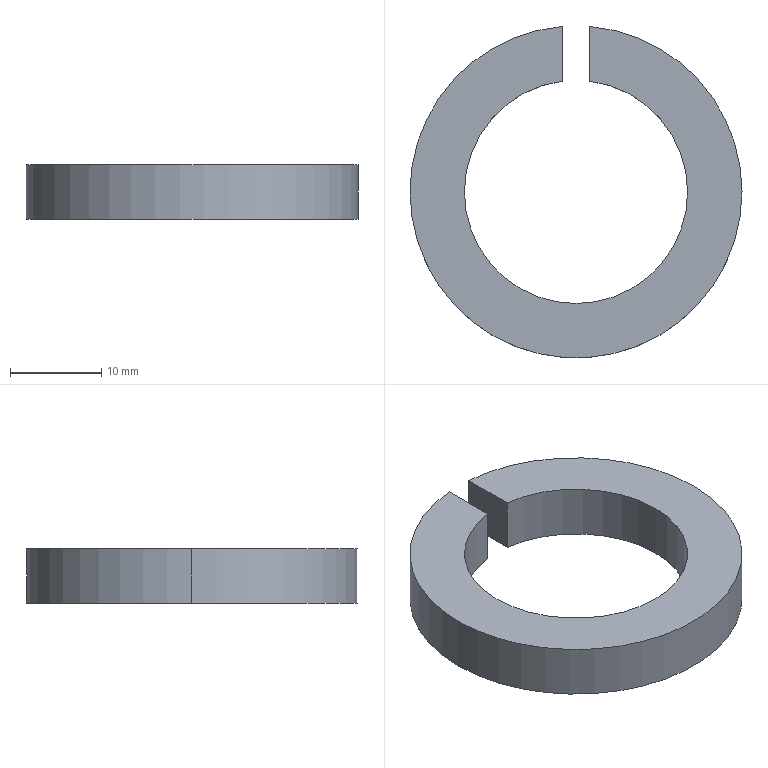Part | STEP file | GB/T 93-1987 standard spring washer (assembly) 24×6 (65Mn) | 1 solid | 10 faces | box 36.439 x 36.377 x 6 mm | volume 3321 mm3 | cylinder 6 | plane 4 | commonest cylinder face diameters 24.5 x3 36.439 x3
STEP:
#1=CARTESIAN_POINT('',(0.,0.,0.));
#2=DIRECTION('',(0.,0.,1.));
#3=DIRECTION('',(1.,0.,0.));
#4=AXIS2_PLACEMENT_3D('',#1,#2,#3);
#5=CARTESIAN_POINT('',(-12.25,0.,6.));
#6=VERTEX_POINT('',#5);
#7=CARTESIAN_POINT('',(-12.25,0.,0.));
#8=VERTEX_POINT('',#7);
#9=CARTESIAN_POINT('',(-12.25,0.,6.));
#10=DIRECTION('',(0.,0.,-1.));
#11=VECTOR('',#10,1.);
#12=LINE('',#9,#11);
#13=CARTESIAN_POINT('',(0.,0.,6.));
#14=DIRECTION('',(0.,0.,-1.));
#15=DIRECTION('',(-1.,0.,0.));
#16=AXIS2_PLACEMENT_3D('',#13,#14,#15);
#17=CYLINDRICAL_SURFACE('',#16,12.25);
#18=CARTESIAN_POINT('',(6.283,0.));
#19=DIRECTION('',(0.,1.));
#20=VECTOR('',#19,1.);
#21=LINE('',#18,#20);
#22=(GEOMETRIC_REPRESENTATION_CONTEXT(2)PARAMETRIC_REPRESENTATION_CONTEXT()REPRESENTATION_CONTEXT('',''));
#23=DEFINITIONAL_REPRESENTATION('',(#21),#22);
#24=PCURVE('',#17,#23);
#25=CARTESIAN_POINT('',(0.,0.,6.));
#26=DIRECTION('',(0.,0.,-1.));
#27=DIRECTION('',(-1.,0.,0.));
#28=AXIS2_PLACEMENT_3D('',#25,#26,#27);
#29=CYLINDRICAL_SURFACE('',#28,12.25);
#30=CARTESIAN_POINT('',(0.,0.));
#31=DIRECTION('',(0.,1.));
#32=VECTOR('',#31,1.);
#33=LINE('',#30,#32);
#34=(GEOMETRIC_REPRESENTATION_CONTEXT(2)PARAMETRIC_REPRESENTATION_CONTEXT()REPRESENTATION_CONTEXT('',''));
#35=DEFINITIONAL_REPRESENTATION('',(#33),#34);
#36=PCURVE('',#29,#35);
#37=SURFACE_CURVE('',#12,(#24,#36),.PCURVE_S1.);
#38=EDGE_CURVE('',#6,#8,#37,.T.);
#39=ORIENTED_EDGE('',*,*,#38,.T.);
#40=CARTESIAN_POINT('',(12.25,0.,0.));
#41=VERTEX_POINT('',#40);
#42=CARTESIAN_POINT('',(0.,0.,0.));
#43=DIRECTION('',(0.,0.,-1.));
#44=DIRECTION('',(1.,0.,0.));
#45=AXIS2_PLACEMENT_3D('',#42,#43,#44);
#46=CIRCLE('',#45,12.25);
#47=CARTESIAN_POINT('',(3.142,6.));
#48=DIRECTION('',(1.,0.));
#49=VECTOR('',#48,1.);
#50=LINE('',#47,#49);
#51=(GEOMETRIC_REPRESENTATION_CONTEXT(2)PARAMETRIC_REPRESENTATION_CONTEXT()REPRESENTATION_CONTEXT('',''));
#52=DEFINITIONAL_REPRESENTATION('',(#50),#51);
#53=PCURVE('',#17,#52);
#54=CARTESIAN_POINT('',(0.,0.,0.));
#55=DIRECTION('',(0.,0.,1.));
#56=DIRECTION('',(1.,0.,0.));
#57=AXIS2_PLACEMENT_3D('',#54,#55,#56);
#58=PLANE('',#57);
#59=CARTESIAN_POINT('',(12.25,0.));
#60=CARTESIAN_POINT('',(12.25,-21.218));
#61=CARTESIAN_POINT('',(-6.125,-10.609));
#62=CARTESIAN_POINT('',(-24.5,0.));
#63=CARTESIAN_POINT('',(-6.125,10.609));
#64=CARTESIAN_POINT('',(12.25,21.218));
#65=CARTESIAN_POINT('',(12.25,0.));
#66=(BOUNDED_CURVE()B_SPLINE_CURVE(2,(#59,#60,#61,#62,#63,#64,#65),.UNSPECIFIED.,.T.,.F.)B_SPLINE_CURVE_WITH_KNOTS((1,2,2,2,2,1),(-2.094,0.,2.094,4.189,6.283,8.378),.UNSPECIFIED.)CURVE()GEOMETRIC_REPRESENTATION_ITEM()RATIONAL_B_SPLINE_CURVE((1.,0.5,1.,0.5,1.,0.5,1.))REPRESENTATION_ITEM(''));
#67=(GEOMETRIC_REPRESENTATION_CONTEXT(2)PARAMETRIC_REPRESENTATION_CONTEXT()REPRESENTATION_CONTEXT('',''));
#68=DEFINITIONAL_REPRESENTATION('',(#66),#67);
#69=PCURVE('',#58,#68);
#70=SURFACE_CURVE('',#46,(#53,#69),.PCURVE_S1.);
#71=EDGE_CURVE('',#41,#8,#70,.T.);
#72=ORIENTED_EDGE('',*,*,#71,.F.);
#73=CARTESIAN_POINT('',(12.25,0.,6.));
#74=VERTEX_POINT('',#73);
#75=CARTESIAN_POINT('',(12.25,0.,6.));
#76=DIRECTION('',(0.,0.,-1.));
#77=VECTOR('',#76,1.);
#78=LINE('',#75,#77);
#79=CARTESIAN_POINT('',(3.142,0.));
#80=DIRECTION('',(0.,1.));
#81=VECTOR('',#80,1.);
#82=LINE('',#79,#81);
#83=(GEOMETRIC_REPRESENTATION_CONTEXT(2)PARAMETRIC_REPRESENTATION_CONTEXT()REPRESENTATION_CONTEXT('',''));
#84=DEFINITIONAL_REPRESENTATION('',(#82),#83);
#85=PCURVE('',#17,#84);
#86=CARTESIAN_POINT('',(0.,0.,6.));
#87=DIRECTION('',(0.,0.,-1.));
#88=DIRECTION('',(-1.,0.,0.));
#89=AXIS2_PLACEMENT_3D('',#86,#87,#88);
#90=CYLINDRICAL_SURFACE('',#89,12.25);
#91=CARTESIAN_POINT('',(3.142,0.));
#92=DIRECTION('',(0.,1.));
#93=VECTOR('',#92,1.);
#94=LINE('',#91,#93);
#95=(GEOMETRIC_REPRESENTATION_CONTEXT(2)PARAMETRIC_REPRESENTATION_CONTEXT()REPRESENTATION_CONTEXT('',''));
#96=DEFINITIONAL_REPRESENTATION('',(#94),#95);
#97=PCURVE('',#90,#96);
#98=SURFACE_CURVE('',#78,(#85,#97),.PCURVE_S1.);
#99=EDGE_CURVE('',#74,#41,#98,.T.);
#100=ORIENTED_EDGE('',*,*,#99,.F.);
#101=CARTESIAN_POINT('',(0.,0.,6.));
#102=DIRECTION('',(0.,0.,-1.));
#103=DIRECTION('',(1.,0.,0.));
#104=AXIS2_PLACEMENT_3D('',#101,#102,#103);
#105=CIRCLE('',#104,12.25);
#106=CARTESIAN_POINT('',(3.142,0.));
#107=DIRECTION('',(1.,0.));
#108=VECTOR('',#107,1.);
#109=LINE('',#106,#108);
#110=(GEOMETRIC_REPRESENTATION_CONTEXT(2)PARAMETRIC_REPRESENTATION_CONTEXT()REPRESENTATION_CONTEXT('',''));
#111=DEFINITIONAL_REPRESENTATION('',(#109),#110);
#112=PCURVE('',#17,#111);
#113=CARTESIAN_POINT('',(0.,0.,6.));
#114=DIRECTION('',(0.,0.,1.));
#115=DIRECTION('',(1.,0.,0.));
#116=AXIS2_PLACEMENT_3D('',#113,#114,#115);
#117=PLANE('',#116);
#118=CARTESIAN_POINT('',(12.25,0.));
#119=CARTESIAN_POINT('',(12.25,-21.218));
#120=CARTESIAN_POINT('',(-6.125,-10.609));
#121=CARTESIAN_POINT('',(-24.5,0.));
#122=CARTESIAN_POINT('',(-6.125,10.609));
#123=CARTESIAN_POINT('',(12.25,21.218));
#124=CARTESIAN_POINT('',(12.25,0.));
#125=(BOUNDED_CURVE()B_SPLINE_CURVE(2,(#118,#119,#120,#121,#122,#123,#124),.UNSPECIFIED.,.T.,.F.)B_SPLINE_CURVE_WITH_KNOTS((1,2,2,2,2,1),(-2.094,0.,2.094,4.189,6.283,8.378),.UNSPECIFIED.)CURVE()GEOMETRIC_REPRESENTATION_ITEM()RATIONAL_B_SPLINE_CURVE((1.,0.5,1.,0.5,1.,0.5,1.))REPRESENTATION_ITEM(''));
#126=(GEOMETRIC_REPRESENTATION_CONTEXT(2)PARAMETRIC_REPRESENTATION_CONTEXT()REPRESENTATION_CONTEXT('',''));
#127=DEFINITIONAL_REPRESENTATION('',(#125),#126);
#128=PCURVE('',#117,#127);
#129=SURFACE_CURVE('',#105,(#112,#128),.PCURVE_S1.);
#130=EDGE_CURVE('',#74,#6,#129,.T.);
#131=ORIENTED_EDGE('',*,*,#130,.T.);
#132=EDGE_LOOP('',(#39,#72,#100,#131));
#133=FACE_BOUND('',#132,.F.);
#134=ADVANCED_FACE('',(#133),#17,.F.);
#135=CARTESIAN_POINT('',(-1.5,12.158,6.));
#136=VERTEX_POINT('',#135);
#137=CARTESIAN_POINT('',(-1.5,12.158,0.));
#138=VERTEX_POINT('',#137);
#139=CARTESIAN_POINT('',(-1.5,12.158,6.));
#140=DIRECTION('',(0.,0.,-1.));
#141=VECTOR('',#140,1.);
#142=LINE('',#139,#141);
#143=CARTESIAN_POINT('',(1.448,0.));
#144=DIRECTION('',(0.,1.));
#145=VECTOR('',#144,1.);
#146=LINE('',#143,#145);
#147=(GEOMETRIC_REPRESENTATION_CONTEXT(2)PARAMETRIC_REPRESENTATION_CONTEXT()REPRESENTATION_CONTEXT('',''));
#148=DEFINITIONAL_REPRESENTATION('',(#146),#147);
#149=PCURVE('',#29,#148);
#150=CARTESIAN_POINT('',(-1.5,18.158,6.));
#151=DIRECTION('',(-1.,0.,0.));
#152=DIRECTION('',(0.,0.,1.));
#153=AXIS2_PLACEMENT_3D('',#150,#151,#152);
#154=PLANE('',#153);
#155=CARTESIAN_POINT('',(0.,-6.));
#156=DIRECTION('',(-1.,0.));
#157=VECTOR('',#156,1.);
#158=LINE('',#155,#157);
#159=(GEOMETRIC_REPRESENTATION_CONTEXT(2)PARAMETRIC_REPRESENTATION_CONTEXT()REPRESENTATION_CONTEXT('',''));
#160=DEFINITIONAL_REPRESENTATION('',(#158),#159);
#161=PCURVE('',#154,#160);
#162=SURFACE_CURVE('',#142,(#149,#161),.PCURVE_S1.);
#163=EDGE_CURVE('',#136,#138,#162,.T.);
#164=ORIENTED_EDGE('',*,*,#163,.T.);
#165=CARTESIAN_POINT('',(0.,0.,0.));
#166=DIRECTION('',(0.,0.,-1.));
#167=DIRECTION('',(1.,0.,0.));
#168=AXIS2_PLACEMENT_3D('',#165,#166,#167);
#169=CIRCLE('',#168,12.25);
#170=CARTESIAN_POINT('',(-3.142,6.));
#171=DIRECTION('',(1.,0.));
#172=VECTOR('',#171,1.);
#173=LINE('',#170,#172);
#174=(GEOMETRIC_REPRESENTATION_CONTEXT(2)PARAMETRIC_REPRESENTATION_CONTEXT()REPRESENTATION_CONTEXT('',''));
#175=DEFINITIONAL_REPRESENTATION('',(#173),#174);
#176=PCURVE('',#29,#175);
#177=CARTESIAN_POINT('',(12.25,0.));
#178=CARTESIAN_POINT('',(12.25,-21.218));
#179=CARTESIAN_POINT('',(-6.125,-10.609));
#180=CARTESIAN_POINT('',(-24.5,0.));
#181=CARTESIAN_POINT('',(-6.125,10.609));
#182=CARTESIAN_POINT('',(12.25,21.218));
#183=CARTESIAN_POINT('',(12.25,0.));
#184=(BOUNDED_CURVE()B_SPLINE_CURVE(2,(#177,#178,#179,#180,#181,#182,#183),.UNSPECIFIED.,.T.,.F.)B_SPLINE_CURVE_WITH_KNOTS((1,2,2,2,2,1),(-2.094,0.,2.094,4.189,6.283,8.378),.UNSPECIFIED.)CURVE()GEOMETRIC_REPRESENTATION_ITEM()RATIONAL_B_SPLINE_CURVE((1.,0.5,1.,0.5,1.,0.5,1.))REPRESENTATION_ITEM(''));
#185=(GEOMETRIC_REPRESENTATION_CONTEXT(2)PARAMETRIC_REPRESENTATION_CONTEXT()REPRESENTATION_CONTEXT('',''));
#186=DEFINITIONAL_REPRESENTATION('',(#184),#185);
#187=PCURVE('',#58,#186);
#188=SURFACE_CURVE('',#169,(#176,#187),.PCURVE_S1.);
#189=EDGE_CURVE('',#8,#138,#188,.T.);
#190=ORIENTED_EDGE('',*,*,#189,.F.);
#191=ORIENTED_EDGE('',*,*,#38,.F.);
#192=CARTESIAN_POINT('',(0.,0.,6.));
#193=DIRECTION('',(0.,0.,-1.));
#194=DIRECTION('',(1.,0.,0.));
#195=AXIS2_PLACEMENT_3D('',#192,#193,#194);
#196=CIRCLE('',#195,12.25);
#197=CARTESIAN_POINT('',(-3.142,0.));
#198=DIRECTION('',(1.,0.));
#199=VECTOR('',#198,1.);
#200=LINE('',#197,#199);
#201=(GEOMETRIC_REPRESENTATION_CONTEXT(2)PARAMETRIC_REPRESENTATION_CONTEXT()REPRESENTATION_CONTEXT('',''));
#202=DEFINITIONAL_REPRESENTATION('',(#200),#201);
#203=PCURVE('',#29,#202);
#204=CARTESIAN_POINT('',(12.25,0.));
#205=CARTESIAN_POINT('',(12.25,-21.218));
#206=CARTESIAN_POINT('',(-6.125,-10.609));
#207=CARTESIAN_POINT('',(-24.5,0.));
#208=CARTESIAN_POINT('',(-6.125,10.609));
#209=CARTESIAN_POINT('',(12.25,21.218));
#210=CARTESIAN_POINT('',(12.25,0.));
#211=(BOUNDED_CURVE()B_SPLINE_CURVE(2,(#204,#205,#206,#207,#208,#209,#210),.UNSPECIFIED.,.T.,.F.)B_SPLINE_CURVE_WITH_KNOTS((1,2,2,2,2,1),(-2.094,0.,2.094,4.189,6.283,8.378),.UNSPECIFIED.)CURVE()GEOMETRIC_REPRESENTATION_ITEM()RATIONAL_B_SPLINE_CURVE((1.,0.5,1.,0.5,1.,0.5,1.))REPRESENTATION_ITEM(''));
#212=(GEOMETRIC_REPRESENTATION_CONTEXT(2)PARAMETRIC_REPRESENTATION_CONTEXT()REPRESENTATION_CONTEXT('',''));
#213=DEFINITIONAL_REPRESENTATION('',(#211),#212);
#214=PCURVE('',#117,#213);
#215=SURFACE_CURVE('',#196,(#203,#214),.PCURVE_S1.);
#216=EDGE_CURVE('',#6,#136,#215,.T.);
#217=ORIENTED_EDGE('',*,*,#216,.T.);
#218=EDGE_LOOP('',(#164,#190,#191,#217));
#219=FACE_BOUND('',#218,.F.);
#220=ADVANCED_FACE('',(#219),#29,.F.);
#221=CARTESIAN_POINT('',(18.22,0.,6.));
#222=VERTEX_POINT('',#221);
#223=CARTESIAN_POINT('',(1.5,18.158,6.));
#224=VERTEX_POINT('',#223);
#225=CARTESIAN_POINT('',(0.,0.,6.));
#226=DIRECTION('',(0.,0.,1.));
#227=DIRECTION('',(1.,0.,0.));
#228=AXIS2_PLACEMENT_3D('',#225,#226,#227);
#229=CIRCLE('',#228,18.22);
#230=CARTESIAN_POINT('',(0.,0.,6.));
#231=DIRECTION('',(0.,0.,-1.));
#232=DIRECTION('',(-1.,0.,0.));
#233=AXIS2_PLACEMENT_3D('',#230,#231,#232);
#234=CYLINDRICAL_SURFACE('',#233,18.22);
#235=CARTESIAN_POINT('',(3.142,0.));
#236=DIRECTION('',(-1.,0.));
#237=VECTOR('',#236,1.);
#238=LINE('',#235,#237);
#239=(GEOMETRIC_REPRESENTATION_CONTEXT(2)PARAMETRIC_REPRESENTATION_CONTEXT()REPRESENTATION_CONTEXT('',''));
#240=DEFINITIONAL_REPRESENTATION('',(#238),#239);
#241=PCURVE('',#234,#240);
#242=CARTESIAN_POINT('',(0.,0.));
#243=DIRECTION('',(1.,0.));
#244=AXIS2_PLACEMENT_2D('',#242,#243);
#245=CIRCLE('',#244,18.22);
#246=(GEOMETRIC_REPRESENTATION_CONTEXT(2)PARAMETRIC_REPRESENTATION_CONTEXT()REPRESENTATION_CONTEXT('',''));
#247=DEFINITIONAL_REPRESENTATION('',(#245),#246);
#248=PCURVE('',#117,#247);
#249=SURFACE_CURVE('',#229,(#241,#248),.PCURVE_S1.);
#250=EDGE_CURVE('',#222,#224,#249,.T.);
#251=ORIENTED_EDGE('',*,*,#250,.F.);
#252=CARTESIAN_POINT('',(18.22,0.,0.));
#253=VERTEX_POINT('',#252);
#254=CARTESIAN_POINT('',(18.22,0.,6.));
#255=DIRECTION('',(0.,0.,-1.));
#256=VECTOR('',#255,1.);
#257=LINE('',#254,#256);
#258=CARTESIAN_POINT('',(3.142,0.));
#259=DIRECTION('',(0.,1.));
#260=VECTOR('',#259,1.);
#261=LINE('',#258,#260);
#262=(GEOMETRIC_REPRESENTATION_CONTEXT(2)PARAMETRIC_REPRESENTATION_CONTEXT()REPRESENTATION_CONTEXT('',''));
#263=DEFINITIONAL_REPRESENTATION('',(#261),#262);
#264=PCURVE('',#234,#263);
#265=CARTESIAN_POINT('',(0.,0.,6.));
#266=DIRECTION('',(0.,0.,-1.));
#267=DIRECTION('',(-1.,0.,0.));
#268=AXIS2_PLACEMENT_3D('',#265,#266,#267);
#269=CYLINDRICAL_SURFACE('',#268,18.22);
#270=CARTESIAN_POINT('',(3.142,0.));
#271=DIRECTION('',(0.,1.));
#272=VECTOR('',#271,1.);
#273=LINE('',#270,#272);
#274=(GEOMETRIC_REPRESENTATION_CONTEXT(2)PARAMETRIC_REPRESENTATION_CONTEXT()REPRESENTATION_CONTEXT('',''));
#275=DEFINITIONAL_REPRESENTATION('',(#273),#274);
#276=PCURVE('',#269,#275);
#277=SURFACE_CURVE('',#257,(#264,#276),.PCURVE_S1.);
#278=EDGE_CURVE('',#222,#253,#277,.T.);
#279=ORIENTED_EDGE('',*,*,#278,.T.);
#280=CARTESIAN_POINT('',(1.5,18.158,0.));
#281=VERTEX_POINT('',#280);
#282=CARTESIAN_POINT('',(0.,0.,0.));
#283=DIRECTION('',(0.,0.,1.));
#284=DIRECTION('',(1.,0.,0.));
#285=AXIS2_PLACEMENT_3D('',#282,#283,#284);
#286=CIRCLE('',#285,18.22);
#287=CARTESIAN_POINT('',(3.142,6.));
#288=DIRECTION('',(-1.,0.));
#289=VECTOR('',#288,1.);
#290=LINE('',#287,#289);
#291=(GEOMETRIC_REPRESENTATION_CONTEXT(2)PARAMETRIC_REPRESENTATION_CONTEXT()REPRESENTATION_CONTEXT('',''));
#292=DEFINITIONAL_REPRESENTATION('',(#290),#291);
#293=PCURVE('',#234,#292);
#294=CARTESIAN_POINT('',(0.,0.));
#295=DIRECTION('',(1.,0.));
#296=AXIS2_PLACEMENT_2D('',#294,#295);
#297=CIRCLE('',#296,18.22);
#298=(GEOMETRIC_REPRESENTATION_CONTEXT(2)PARAMETRIC_REPRESENTATION_CONTEXT()REPRESENTATION_CONTEXT('',''));
#299=DEFINITIONAL_REPRESENTATION('',(#297),#298);
#300=PCURVE('',#58,#299);
#301=SURFACE_CURVE('',#286,(#293,#300),.PCURVE_S1.);
#302=EDGE_CURVE('',#253,#281,#301,.T.);
#303=ORIENTED_EDGE('',*,*,#302,.T.);
#304=CARTESIAN_POINT('',(1.5,18.158,6.));
#305=DIRECTION('',(0.,0.,-1.));
#306=VECTOR('',#305,1.);
#307=LINE('',#304,#306);
#308=CARTESIAN_POINT('',(1.653,0.));
#309=DIRECTION('',(0.,1.));
#310=VECTOR('',#309,1.);
#311=LINE('',#308,#310);
#312=(GEOMETRIC_REPRESENTATION_CONTEXT(2)PARAMETRIC_REPRESENTATION_CONTEXT()REPRESENTATION_CONTEXT('',''));
#313=DEFINITIONAL_REPRESENTATION('',(#311),#312);
#314=PCURVE('',#234,#313);
#315=CARTESIAN_POINT('',(1.5,18.158,6.));
#316=DIRECTION('',(1.,0.,0.));
#317=DIRECTION('',(0.,0.,-1.));
#318=AXIS2_PLACEMENT_3D('',#315,#316,#317);
#319=PLANE('',#318);
#320=CARTESIAN_POINT('',(0.,0.));
#321=DIRECTION('',(1.,0.));
#322=VECTOR('',#321,1.);
#323=LINE('',#320,#322);
#324=(GEOMETRIC_REPRESENTATION_CONTEXT(2)PARAMETRIC_REPRESENTATION_CONTEXT()REPRESENTATION_CONTEXT('',''));
#325=DEFINITIONAL_REPRESENTATION('',(#323),#324);
#326=PCURVE('',#319,#325);
#327=SURFACE_CURVE('',#307,(#314,#326),.PCURVE_S1.);
#328=EDGE_CURVE('',#224,#281,#327,.T.);
#329=ORIENTED_EDGE('',*,*,#328,.F.);
#330=EDGE_LOOP('',(#251,#279,#303,#329));
#331=FACE_BOUND('',#330,.T.);
#332=ADVANCED_FACE('',(#331),#234,.T.);
#333=ORIENTED_EDGE('',*,*,#278,.F.);
#334=CARTESIAN_POINT('',(-18.22,0.,6.));
#335=VERTEX_POINT('',#334);
#336=CARTESIAN_POINT('',(0.,0.,6.));
#337=DIRECTION('',(0.,0.,1.));
#338=DIRECTION('',(1.,0.,0.));
#339=AXIS2_PLACEMENT_3D('',#336,#337,#338);
#340=CIRCLE('',#339,18.22);
#341=CARTESIAN_POINT('',(9.425,0.));
#342=DIRECTION('',(-1.,0.));
#343=VECTOR('',#342,1.);
#344=LINE('',#341,#343);
#345=(GEOMETRIC_REPRESENTATION_CONTEXT(2)PARAMETRIC_REPRESENTATION_CONTEXT()REPRESENTATION_CONTEXT('',''));
#346=DEFINITIONAL_REPRESENTATION('',(#344),#345);
#347=PCURVE('',#269,#346);
#348=CARTESIAN_POINT('',(0.,0.));
#349=DIRECTION('',(1.,0.));
#350=AXIS2_PLACEMENT_2D('',#348,#349);
#351=CIRCLE('',#350,18.22);
#352=(GEOMETRIC_REPRESENTATION_CONTEXT(2)PARAMETRIC_REPRESENTATION_CONTEXT()REPRESENTATION_CONTEXT('',''));
#353=DEFINITIONAL_REPRESENTATION('',(#351),#352);
#354=PCURVE('',#117,#353);
#355=SURFACE_CURVE('',#340,(#347,#354),.PCURVE_S1.);
#356=EDGE_CURVE('',#335,#222,#355,.T.);
#357=ORIENTED_EDGE('',*,*,#356,.F.);
#358=CARTESIAN_POINT('',(-18.22,0.,0.));
#359=VERTEX_POINT('',#358);
#360=CARTESIAN_POINT('',(-18.22,0.,6.));
#361=DIRECTION('',(0.,0.,-1.));
#362=VECTOR('',#361,1.);
#363=LINE('',#360,#362);
#364=CARTESIAN_POINT('',(6.283,0.));
#365=DIRECTION('',(0.,1.));
#366=VECTOR('',#365,1.);
#367=LINE('',#364,#366);
#368=(GEOMETRIC_REPRESENTATION_CONTEXT(2)PARAMETRIC_REPRESENTATION_CONTEXT()REPRESENTATION_CONTEXT('',''));
#369=DEFINITIONAL_REPRESENTATION('',(#367),#368);
#370=PCURVE('',#269,#369);
#371=CARTESIAN_POINT('',(0.,0.,6.));
#372=DIRECTION('',(0.,0.,-1.));
#373=DIRECTION('',(-1.,0.,0.));
#374=AXIS2_PLACEMENT_3D('',#371,#372,#373);
#375=CYLINDRICAL_SURFACE('',#374,18.22);
#376=CARTESIAN_POINT('',(0.,0.));
#377=DIRECTION('',(0.,1.));
#378=VECTOR('',#377,1.);
#379=LINE('',#376,#378);
#380=(GEOMETRIC_REPRESENTATION_CONTEXT(2)PARAMETRIC_REPRESENTATION_CONTEXT()REPRESENTATION_CONTEXT('',''));
#381=DEFINITIONAL_REPRESENTATION('',(#379),#380);
#382=PCURVE('',#375,#381);
#383=SURFACE_CURVE('',#363,(#370,#382),.PCURVE_S1.);
#384=EDGE_CURVE('',#335,#359,#383,.T.);
#385=ORIENTED_EDGE('',*,*,#384,.T.);
#386=CARTESIAN_POINT('',(0.,0.,0.));
#387=DIRECTION('',(0.,0.,1.));
#388=DIRECTION('',(1.,0.,0.));
#389=AXIS2_PLACEMENT_3D('',#386,#387,#388);
#390=CIRCLE('',#389,18.22);
#391=CARTESIAN_POINT('',(9.425,6.));
#392=DIRECTION('',(-1.,0.));
#393=VECTOR('',#392,1.);
#394=LINE('',#391,#393);
#395=(GEOMETRIC_REPRESENTATION_CONTEXT(2)PARAMETRIC_REPRESENTATION_CONTEXT()REPRESENTATION_CONTEXT('',''));
#396=DEFINITIONAL_REPRESENTATION('',(#394),#395);
#397=PCURVE('',#269,#396);
#398=CARTESIAN_POINT('',(0.,0.));
#399=DIRECTION('',(1.,0.));
#400=AXIS2_PLACEMENT_2D('',#398,#399);
#401=CIRCLE('',#400,18.22);
#402=(GEOMETRIC_REPRESENTATION_CONTEXT(2)PARAMETRIC_REPRESENTATION_CONTEXT()REPRESENTATION_CONTEXT('',''));
#403=DEFINITIONAL_REPRESENTATION('',(#401),#402);
#404=PCURVE('',#58,#403);
#405=SURFACE_CURVE('',#390,(#397,#404),.PCURVE_S1.);
#406=EDGE_CURVE('',#359,#253,#405,.T.);
#407=ORIENTED_EDGE('',*,*,#406,.T.);
#408=EDGE_LOOP('',(#333,#357,#385,#407));
#409=FACE_BOUND('',#408,.T.);
#410=ADVANCED_FACE('',(#409),#269,.T.);
#411=ORIENTED_EDGE('',*,*,#384,.F.);
#412=CARTESIAN_POINT('',(-1.5,18.158,6.));
#413=VERTEX_POINT('',#412);
#414=CARTESIAN_POINT('',(0.,0.,6.));
#415=DIRECTION('',(0.,0.,1.));
#416=DIRECTION('',(1.,0.,0.));
#417=AXIS2_PLACEMENT_3D('',#414,#415,#416);
#418=CIRCLE('',#417,18.22);
#419=CARTESIAN_POINT('',(3.142,0.));
#420=DIRECTION('',(-1.,0.));
#421=VECTOR('',#420,1.);
#422=LINE('',#419,#421);
#423=(GEOMETRIC_REPRESENTATION_CONTEXT(2)PARAMETRIC_REPRESENTATION_CONTEXT()REPRESENTATION_CONTEXT('',''));
#424=DEFINITIONAL_REPRESENTATION('',(#422),#423);
#425=PCURVE('',#375,#424);
#426=CARTESIAN_POINT('',(0.,0.));
#427=DIRECTION('',(1.,0.));
#428=AXIS2_PLACEMENT_2D('',#426,#427);
#429=CIRCLE('',#428,18.22);
#430=(GEOMETRIC_REPRESENTATION_CONTEXT(2)PARAMETRIC_REPRESENTATION_CONTEXT()REPRESENTATION_CONTEXT('',''));
#431=DEFINITIONAL_REPRESENTATION('',(#429),#430);
#432=PCURVE('',#117,#431);
#433=SURFACE_CURVE('',#418,(#425,#432),.PCURVE_S1.);
#434=EDGE_CURVE('',#413,#335,#433,.T.);
#435=ORIENTED_EDGE('',*,*,#434,.F.);
#436=CARTESIAN_POINT('',(-1.5,18.158,0.));
#437=VERTEX_POINT('',#436);
#438=CARTESIAN_POINT('',(-1.5,18.158,6.));
#439=DIRECTION('',(0.,0.,-1.));
#440=VECTOR('',#439,1.);
#441=LINE('',#438,#440);
#442=CARTESIAN_POINT('',(1.488,0.));
#443=DIRECTION('',(0.,1.));
#444=VECTOR('',#443,1.);
#445=LINE('',#442,#444);
#446=(GEOMETRIC_REPRESENTATION_CONTEXT(2)PARAMETRIC_REPRESENTATION_CONTEXT()REPRESENTATION_CONTEXT('',''));
#447=DEFINITIONAL_REPRESENTATION('',(#445),#446);
#448=PCURVE('',#375,#447);
#449=CARTESIAN_POINT('',(0.,0.));
#450=DIRECTION('',(-1.,0.));
#451=VECTOR('',#450,1.);
#452=LINE('',#449,#451);
#453=(GEOMETRIC_REPRESENTATION_CONTEXT(2)PARAMETRIC_REPRESENTATION_CONTEXT()REPRESENTATION_CONTEXT('',''));
#454=DEFINITIONAL_REPRESENTATION('',(#452),#453);
#455=PCURVE('',#154,#454);
#456=SURFACE_CURVE('',#441,(#448,#455),.PCURVE_S1.);
#457=EDGE_CURVE('',#413,#437,#456,.T.);
#458=ORIENTED_EDGE('',*,*,#457,.T.);
#459=CARTESIAN_POINT('',(0.,0.,0.));
#460=DIRECTION('',(0.,0.,1.));
#461=DIRECTION('',(1.,0.,0.));
#462=AXIS2_PLACEMENT_3D('',#459,#460,#461);
#463=CIRCLE('',#462,18.22);
#464=CARTESIAN_POINT('',(3.142,6.));
#465=DIRECTION('',(-1.,0.));
#466=VECTOR('',#465,1.);
#467=LINE('',#464,#466);
#468=(GEOMETRIC_REPRESENTATION_CONTEXT(2)PARAMETRIC_REPRESENTATION_CONTEXT()REPRESENTATION_CONTEXT('',''));
#469=DEFINITIONAL_REPRESENTATION('',(#467),#468);
#470=PCURVE('',#375,#469);
#471=CARTESIAN_POINT('',(0.,0.));
#472=DIRECTION('',(1.,0.));
#473=AXIS2_PLACEMENT_2D('',#471,#472);
#474=CIRCLE('',#473,18.22);
#475=(GEOMETRIC_REPRESENTATION_CONTEXT(2)PARAMETRIC_REPRESENTATION_CONTEXT()REPRESENTATION_CONTEXT('',''));
#476=DEFINITIONAL_REPRESENTATION('',(#474),#475);
#477=PCURVE('',#58,#476);
#478=SURFACE_CURVE('',#463,(#470,#477),.PCURVE_S1.);
#479=EDGE_CURVE('',#437,#359,#478,.T.);
#480=ORIENTED_EDGE('',*,*,#479,.T.);
#481=EDGE_LOOP('',(#411,#435,#458,#480));
#482=FACE_BOUND('',#481,.T.);
#483=ADVANCED_FACE('',(#482),#375,.T.);
#484=CARTESIAN_POINT('',(1.5,12.158,0.));
#485=VERTEX_POINT('',#484);
#486=CARTESIAN_POINT('',(1.5,18.158,0.));
#487=DIRECTION('',(0.,-1.,0.));
#488=VECTOR('',#487,1.);
#489=LINE('',#486,#488);
#490=CARTESIAN_POINT('',(6.,0.));
#491=DIRECTION('',(0.,-1.));
#492=VECTOR('',#491,1.);
#493=LINE('',#490,#492);
#494=(GEOMETRIC_REPRESENTATION_CONTEXT(2)PARAMETRIC_REPRESENTATION_CONTEXT()REPRESENTATION_CONTEXT('',''));
#495=DEFINITIONAL_REPRESENTATION('',(#493),#494);
#496=PCURVE('',#319,#495);
#497=CARTESIAN_POINT('',(1.5,18.158));
#498=DIRECTION('',(0.,-1.));
#499=VECTOR('',#498,1.);
#500=LINE('',#497,#499);
#501=(GEOMETRIC_REPRESENTATION_CONTEXT(2)PARAMETRIC_REPRESENTATION_CONTEXT()REPRESENTATION_CONTEXT('',''));
#502=DEFINITIONAL_REPRESENTATION('',(#500),#501);
#503=PCURVE('',#58,#502);
#504=SURFACE_CURVE('',#489,(#496,#503),.PCURVE_S1.);
#505=EDGE_CURVE('',#281,#485,#504,.T.);
#506=ORIENTED_EDGE('',*,*,#505,.T.);
#507=CARTESIAN_POINT('',(1.5,12.158,6.));
#508=VERTEX_POINT('',#507);
#509=CARTESIAN_POINT('',(1.5,12.158,6.));
#510=DIRECTION('',(0.,0.,-1.));
#511=VECTOR('',#510,1.);
#512=LINE('',#509,#511);
#513=CARTESIAN_POINT('',(0.,-6.));
#514=DIRECTION('',(1.,0.));
#515=VECTOR('',#514,1.);
#516=LINE('',#513,#515);
#517=(GEOMETRIC_REPRESENTATION_CONTEXT(2)PARAMETRIC_REPRESENTATION_CONTEXT()REPRESENTATION_CONTEXT('',''));
#518=DEFINITIONAL_REPRESENTATION('',(#516),#517);
#519=PCURVE('',#319,#518);
#520=CARTESIAN_POINT('',(1.694,0.));
#521=DIRECTION('',(0.,1.));
#522=VECTOR('',#521,1.);
#523=LINE('',#520,#522);
#524=(GEOMETRIC_REPRESENTATION_CONTEXT(2)PARAMETRIC_REPRESENTATION_CONTEXT()REPRESENTATION_CONTEXT('',''));
#525=DEFINITIONAL_REPRESENTATION('',(#523),#524);
#526=PCURVE('',#90,#525);
#527=SURFACE_CURVE('',#512,(#519,#526),.PCURVE_S1.);
#528=EDGE_CURVE('',#508,#485,#527,.T.);
#529=ORIENTED_EDGE('',*,*,#528,.F.);
#530=CARTESIAN_POINT('',(1.5,18.158,6.));
#531=DIRECTION('',(0.,-1.,0.));
#532=VECTOR('',#531,1.);
#533=LINE('',#530,#532);
#534=CARTESIAN_POINT('',(0.,0.));
#535=DIRECTION('',(0.,-1.));
#536=VECTOR('',#535,1.);
#537=LINE('',#534,#536);
#538=(GEOMETRIC_REPRESENTATION_CONTEXT(2)PARAMETRIC_REPRESENTATION_CONTEXT()REPRESENTATION_CONTEXT('',''));
#539=DEFINITIONAL_REPRESENTATION('',(#537),#538);
#540=PCURVE('',#319,#539);
#541=CARTESIAN_POINT('',(1.5,18.158));
#542=DIRECTION('',(0.,-1.));
#543=VECTOR('',#542,1.);
#544=LINE('',#541,#543);
#545=(GEOMETRIC_REPRESENTATION_CONTEXT(2)PARAMETRIC_REPRESENTATION_CONTEXT()REPRESENTATION_CONTEXT('',''));
#546=DEFINITIONAL_REPRESENTATION('',(#544),#545);
#547=PCURVE('',#117,#546);
#548=SURFACE_CURVE('',#533,(#540,#547),.PCURVE_S1.);
#549=EDGE_CURVE('',#224,#508,#548,.T.);
#550=ORIENTED_EDGE('',*,*,#549,.F.);
#551=ORIENTED_EDGE('',*,*,#328,.T.);
#552=EDGE_LOOP('',(#506,#529,#550,#551));
#553=FACE_BOUND('',#552,.T.);
#554=ADVANCED_FACE('',(#553),#319,.F.);
#555=CARTESIAN_POINT('',(0.,0.,0.));
#556=DIRECTION('',(0.,0.,-1.));
#557=DIRECTION('',(1.,0.,0.));
#558=AXIS2_PLACEMENT_3D('',#555,#556,#557);
#559=CIRCLE('',#558,12.25);
#560=CARTESIAN_POINT('',(-3.142,6.));
#561=DIRECTION('',(1.,0.));
#562=VECTOR('',#561,1.);
#563=LINE('',#560,#562);
#564=(GEOMETRIC_REPRESENTATION_CONTEXT(2)PARAMETRIC_REPRESENTATION_CONTEXT()REPRESENTATION_CONTEXT('',''));
#565=DEFINITIONAL_REPRESENTATION('',(#563),#564);
#566=PCURVE('',#90,#565);
#567=CARTESIAN_POINT('',(12.25,0.));
#568=CARTESIAN_POINT('',(12.25,-21.218));
#569=CARTESIAN_POINT('',(-6.125,-10.609));
#570=CARTESIAN_POINT('',(-24.5,0.));
#571=CARTESIAN_POINT('',(-6.125,10.609));
#572=CARTESIAN_POINT('',(12.25,21.218));
#573=CARTESIAN_POINT('',(12.25,0.));
#574=(BOUNDED_CURVE()B_SPLINE_CURVE(2,(#567,#568,#569,#570,#571,#572,#573),.UNSPECIFIED.,.T.,.F.)B_SPLINE_CURVE_WITH_KNOTS((1,2,2,2,2,1),(-2.094,0.,2.094,4.189,6.283,8.378),.UNSPECIFIED.)CURVE()GEOMETRIC_REPRESENTATION_ITEM()RATIONAL_B_SPLINE_CURVE((1.,0.5,1.,0.5,1.,0.5,1.))REPRESENTATION_ITEM(''));
#575=(GEOMETRIC_REPRESENTATION_CONTEXT(2)PARAMETRIC_REPRESENTATION_CONTEXT()REPRESENTATION_CONTEXT('',''));
#576=DEFINITIONAL_REPRESENTATION('',(#574),#575);
#577=PCURVE('',#58,#576);
#578=SURFACE_CURVE('',#559,(#566,#577),.PCURVE_S1.);
#579=EDGE_CURVE('',#485,#41,#578,.T.);
#580=ORIENTED_EDGE('',*,*,#579,.F.);
#581=ORIENTED_EDGE('',*,*,#528,.F.);
#582=CARTESIAN_POINT('',(0.,0.,6.));
#583=DIRECTION('',(0.,0.,-1.));
#584=DIRECTION('',(1.,0.,0.));
#585=AXIS2_PLACEMENT_3D('',#582,#583,#584);
#586=CIRCLE('',#585,12.25);
#587=CARTESIAN_POINT('',(-3.142,0.));
#588=DIRECTION('',(1.,0.));
#589=VECTOR('',#588,1.);
#590=LINE('',#587,#589);
#591=(GEOMETRIC_REPRESENTATION_CONTEXT(2)PARAMETRIC_REPRESENTATION_CONTEXT()REPRESENTATION_CONTEXT('',''));
#592=DEFINITIONAL_REPRESENTATION('',(#590),#591);
#593=PCURVE('',#90,#592);
#594=CARTESIAN_POINT('',(12.25,0.));
#595=CARTESIAN_POINT('',(12.25,-21.218));
#596=CARTESIAN_POINT('',(-6.125,-10.609));
#597=CARTESIAN_POINT('',(-24.5,0.));
#598=CARTESIAN_POINT('',(-6.125,10.609));
#599=CARTESIAN_POINT('',(12.25,21.218));
#600=CARTESIAN_POINT('',(12.25,0.));
#601=(BOUNDED_CURVE()B_SPLINE_CURVE(2,(#594,#595,#596,#597,#598,#599,#600),.UNSPECIFIED.,.T.,.F.)B_SPLINE_CURVE_WITH_KNOTS((1,2,2,2,2,1),(-2.094,0.,2.094,4.189,6.283,8.378),.UNSPECIFIED.)CURVE()GEOMETRIC_REPRESENTATION_ITEM()RATIONAL_B_SPLINE_CURVE((1.,0.5,1.,0.5,1.,0.5,1.))REPRESENTATION_ITEM(''));
#602=(GEOMETRIC_REPRESENTATION_CONTEXT(2)PARAMETRIC_REPRESENTATION_CONTEXT()REPRESENTATION_CONTEXT('',''));
#603=DEFINITIONAL_REPRESENTATION('',(#601),#602);
#604=PCURVE('',#117,#603);
#605=SURFACE_CURVE('',#586,(#593,#604),.PCURVE_S1.);
#606=EDGE_CURVE('',#508,#74,#605,.T.);
#607=ORIENTED_EDGE('',*,*,#606,.T.);
#608=ORIENTED_EDGE('',*,*,#99,.T.);
#609=EDGE_LOOP('',(#580,#581,#607,#608));
#610=FACE_BOUND('',#609,.F.);
#611=ADVANCED_FACE('',(#610),#90,.F.);
#612=CARTESIAN_POINT('',(-1.5,18.158,0.));
#613=DIRECTION('',(0.,1.,0.));
#614=VECTOR('',#613,1.);
#615=LINE('',#612,#614);
#616=CARTESIAN_POINT('',(-6.,0.));
#617=DIRECTION('',(0.,1.));
#618=VECTOR('',#617,1.);
#619=LINE('',#616,#618);
#620=(GEOMETRIC_REPRESENTATION_CONTEXT(2)PARAMETRIC_REPRESENTATION_CONTEXT()REPRESENTATION_CONTEXT('',''));
#621=DEFINITIONAL_REPRESENTATION('',(#619),#620);
#622=PCURVE('',#154,#621);
#623=CARTESIAN_POINT('',(-1.5,18.158));
#624=DIRECTION('',(0.,1.));
#625=VECTOR('',#624,1.);
#626=LINE('',#623,#625);
#627=(GEOMETRIC_REPRESENTATION_CONTEXT(2)PARAMETRIC_REPRESENTATION_CONTEXT()REPRESENTATION_CONTEXT('',''));
#628=DEFINITIONAL_REPRESENTATION('',(#626),#627);
#629=PCURVE('',#58,#628);
#630=SURFACE_CURVE('',#615,(#622,#629),.PCURVE_S1.);
#631=EDGE_CURVE('',#138,#437,#630,.T.);
#632=ORIENTED_EDGE('',*,*,#631,.T.);
#633=ORIENTED_EDGE('',*,*,#457,.F.);
#634=CARTESIAN_POINT('',(-1.5,18.158,6.));
#635=DIRECTION('',(0.,1.,0.));
#636=VECTOR('',#635,1.);
#637=LINE('',#634,#636);
#638=CARTESIAN_POINT('',(0.,0.));
#639=DIRECTION('',(0.,1.));
#640=VECTOR('',#639,1.);
#641=LINE('',#638,#640);
#642=(GEOMETRIC_REPRESENTATION_CONTEXT(2)PARAMETRIC_REPRESENTATION_CONTEXT()REPRESENTATION_CONTEXT('',''));
#643=DEFINITIONAL_REPRESENTATION('',(#641),#642);
#644=PCURVE('',#154,#643);
#645=CARTESIAN_POINT('',(-1.5,18.158));
#646=DIRECTION('',(0.,1.));
#647=VECTOR('',#646,1.);
#648=LINE('',#645,#647);
#649=(GEOMETRIC_REPRESENTATION_CONTEXT(2)PARAMETRIC_REPRESENTATION_CONTEXT()REPRESENTATION_CONTEXT('',''));
#650=DEFINITIONAL_REPRESENTATION('',(#648),#649);
#651=PCURVE('',#117,#650);
#652=SURFACE_CURVE('',#637,(#644,#651),.PCURVE_S1.);
#653=EDGE_CURVE('',#136,#413,#652,.T.);
#654=ORIENTED_EDGE('',*,*,#653,.F.);
#655=ORIENTED_EDGE('',*,*,#163,.T.);
#656=EDGE_LOOP('',(#632,#633,#654,#655));
#657=FACE_BOUND('',#656,.T.);
#658=ADVANCED_FACE('',(#657),#154,.F.);
#659=ORIENTED_EDGE('',*,*,#434,.T.);
#660=ORIENTED_EDGE('',*,*,#356,.T.);
#661=ORIENTED_EDGE('',*,*,#250,.T.);
#662=ORIENTED_EDGE('',*,*,#549,.T.);
#663=ORIENTED_EDGE('',*,*,#606,.T.);
#664=ORIENTED_EDGE('',*,*,#130,.T.);
#665=ORIENTED_EDGE('',*,*,#216,.T.);
#666=ORIENTED_EDGE('',*,*,#653,.T.);
#667=EDGE_LOOP('',(#659,#660,#661,#662,#663,#664,#665,#666));
#668=FACE_BOUND('',#667,.T.);
#669=ADVANCED_FACE('',(#668),#117,.T.);
#670=ORIENTED_EDGE('',*,*,#479,.F.);
#671=ORIENTED_EDGE('',*,*,#631,.F.);
#672=ORIENTED_EDGE('',*,*,#189,.F.);
#673=ORIENTED_EDGE('',*,*,#71,.F.);
#674=ORIENTED_EDGE('',*,*,#579,.F.);
#675=ORIENTED_EDGE('',*,*,#505,.F.);
#676=ORIENTED_EDGE('',*,*,#302,.F.);
#677=ORIENTED_EDGE('',*,*,#406,.F.);
#678=EDGE_LOOP('',(#670,#671,#672,#673,#674,#675,#676,#677));
#679=FACE_BOUND('',#678,.T.);
#680=ADVANCED_FACE('',(#679),#58,.F.);
#681=CLOSED_SHELL('',(#134,#220,#332,#410,#483,#554,#611,#658,#669,#680));
#682=MANIFOLD_SOLID_BREP('',#681);
#683=(LENGTH_UNIT()NAMED_UNIT(*)SI_UNIT(.MILLI.,.METRE.));
#684=UNCERTAINTY_MEASURE_WITH_UNIT(LENGTH_MEASURE(0.0000001),#683,'','');
#685=(NAMED_UNIT(*)PLANE_ANGLE_UNIT()SI_UNIT($,.RADIAN.));
#686=(NAMED_UNIT(*)SI_UNIT($,.STERADIAN.)SOLID_ANGLE_UNIT());
#687=(GEOMETRIC_REPRESENTATION_CONTEXT(3)GLOBAL_UNCERTAINTY_ASSIGNED_CONTEXT((#684))GLOBAL_UNIT_ASSIGNED_CONTEXT((#683,#685,#686))REPRESENTATION_CONTEXT('',''));
#688=ADVANCED_BREP_SHAPE_REPRESENTATION('',(#4,#682),#687);